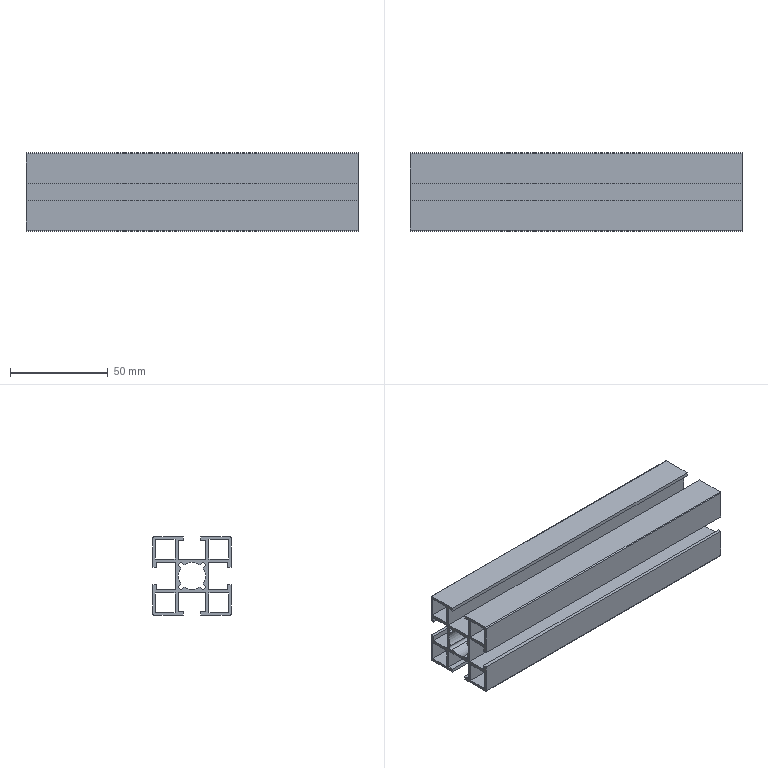Part | 1 solid | 77 faces | box 170 x 40 x 40 mm | volume 67386 mm3 | plane 62 | cylinder 15 | commonest cylinder face diameters 2.2 x6 14 x5 1 x4